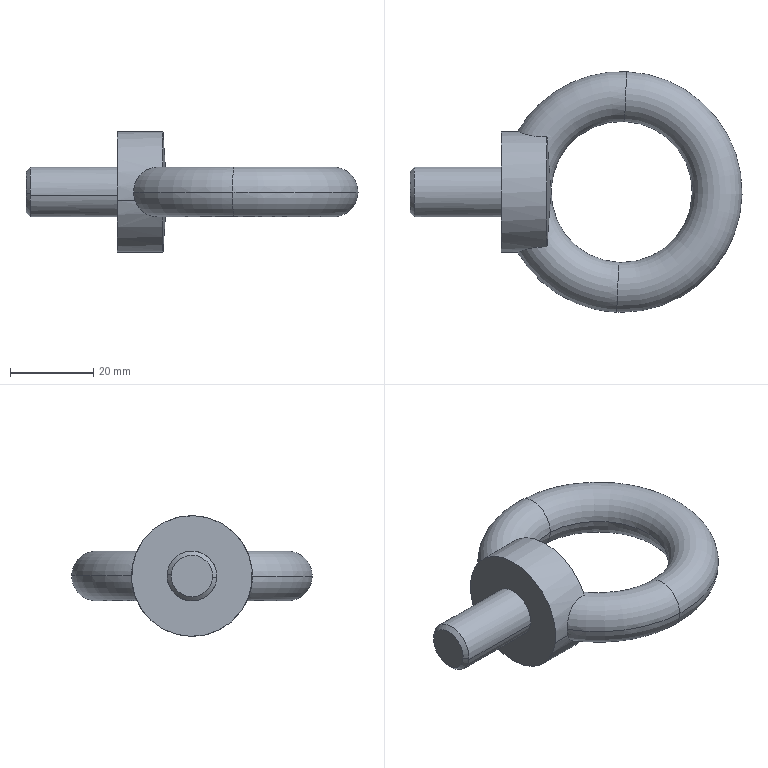Part | STEP file | Positioning_id1086_x_t | 1 solid | 14 faces | box 80 x 58 x 29.1 mm | volume 23470 mm3 | cone 4 | cylinder 4 | torus 4 | plane 2 | commonest cylinder face diameters 12 x2 29.1 x2